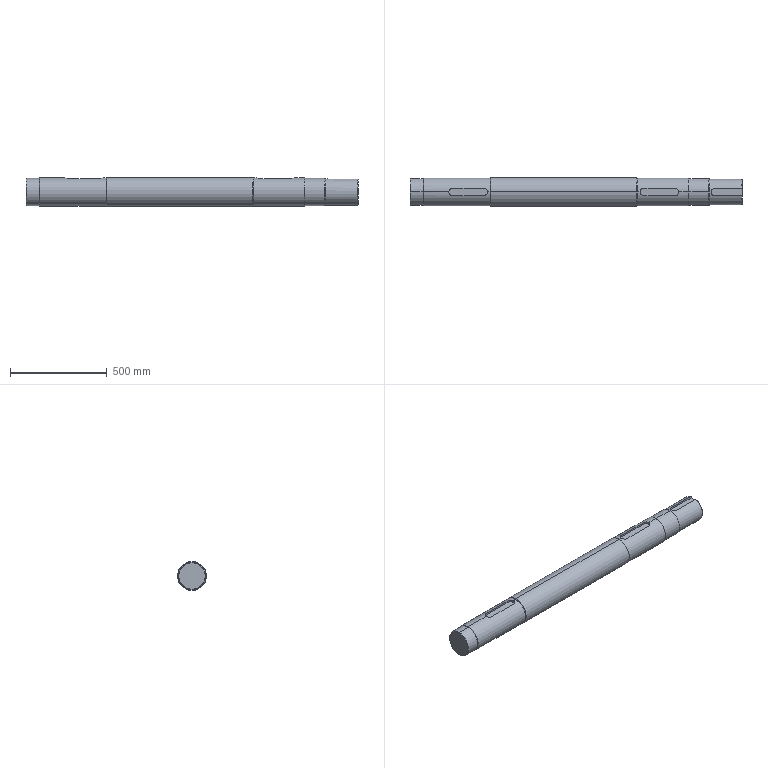Part | SolidWorks | features ICE 2, Chamfer 1, Revolution 1 | 1 solid | 48 faces | box 1719 x 150 x 150 mm | volume 28459508 mm3 | cylinder 19 | plane 16 | cone 13 | commonest cylinder face diameters 40 x6 140 x4 145 x4 135 x2 150 x2 36 x1